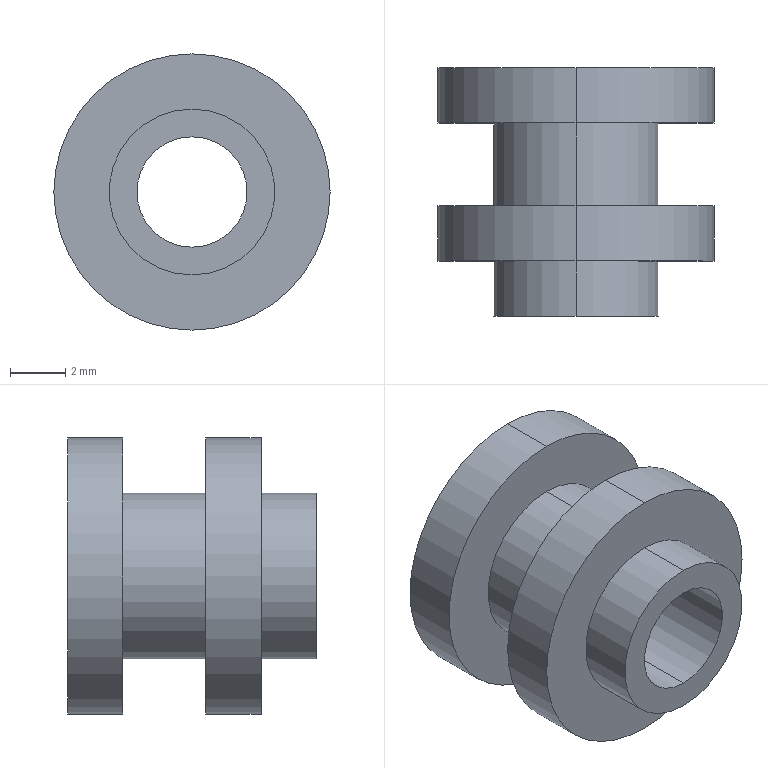Part | SolidWorks | features Extrusion 1, ICE 1, RevCut 1 | 1 solid | 15 faces | box 10 x 9 x 10 mm | volume 342.434 mm3 | cylinder 10 | plane 5 | commonest cylinder face diameters 6 x4 10 x4 4 x2
STEP:
#1=CARTESIAN_POINT('',(0.,0.,-2.));
#2=VERTEX_POINT('',#1);
#3=CARTESIAN_POINT('',(0.,0.,2.));
#4=VERTEX_POINT('',#3);
#5=CARTESIAN_POINT('',(0.,0.,0.));
#6=DIRECTION('',(0.,1.,0.));
#7=DIRECTION('',(0.,0.,1.));
#8=AXIS2_PLACEMENT_3D('',#5,#6,#7);
#9=CIRCLE('',#8,2.);
#10=EDGE_CURVE('',#2,#4,#9,.T.);
#11=ORIENTED_EDGE('',*,*,#10,.F.);
#12=CARTESIAN_POINT('',(0.,9.,-2.));
#13=VERTEX_POINT('',#12);
#14=CARTESIAN_POINT('',(0.,0.,-2.));
#15=DIRECTION('',(0.,1.,0.));
#16=VECTOR('',#15,1000.);
#17=LINE('',#14,#16);
#18=EDGE_CURVE('',#2,#13,#17,.T.);
#19=ORIENTED_EDGE('',*,*,#18,.T.);
#20=CARTESIAN_POINT('',(0.,9.,2.));
#21=VERTEX_POINT('',#20);
#22=CARTESIAN_POINT('',(0.,9.,0.));
#23=DIRECTION('',(0.,1.,0.));
#24=DIRECTION('',(0.,0.,1.));
#25=AXIS2_PLACEMENT_3D('',#22,#23,#24);
#26=CIRCLE('',#25,2.);
#27=EDGE_CURVE('',#13,#21,#26,.T.);
#28=ORIENTED_EDGE('',*,*,#27,.T.);
#29=CARTESIAN_POINT('',(0.,0.,2.));
#30=DIRECTION('',(0.,1.,0.));
#31=VECTOR('',#30,1000.);
#32=LINE('',#29,#31);
#33=EDGE_CURVE('',#4,#21,#32,.T.);
#34=ORIENTED_EDGE('',*,*,#33,.F.);
#35=EDGE_LOOP('',(#11,#19,#28,#34));
#36=FACE_OUTER_BOUND('',#35,.T.);
#37=CARTESIAN_POINT('',(0.,0.,0.));
#38=DIRECTION('',(0.,1.,0.));
#39=DIRECTION('',(0.,0.,1.));
#40=AXIS2_PLACEMENT_3D('',#37,#38,#39);
#41=CYLINDRICAL_SURFACE('',#40,2.);
#42=ADVANCED_FACE('',(#36),#41,.F.);
#43=CARTESIAN_POINT('',(0.,2.,-3.));
#44=VERTEX_POINT('',#43);
#45=CARTESIAN_POINT('',(0.,2.,3.));
#46=VERTEX_POINT('',#45);
#47=CARTESIAN_POINT('',(0.,2.,0.));
#48=DIRECTION('',(0.,-1.,0.));
#49=DIRECTION('',(0.,0.,-1.));
#50=AXIS2_PLACEMENT_3D('',#47,#48,#49);
#51=CIRCLE('',#50,3.);
#52=EDGE_CURVE('',#44,#46,#51,.T.);
#53=ORIENTED_EDGE('',*,*,#52,.T.);
#54=CARTESIAN_POINT('',(0.,0.,3.));
#55=VERTEX_POINT('',#54);
#56=CARTESIAN_POINT('',(0.,0.,3.));
#57=DIRECTION('',(0.,-1.,0.));
#58=VECTOR('',#57,1000.);
#59=LINE('',#56,#58);
#60=EDGE_CURVE('',#46,#55,#59,.T.);
#61=ORIENTED_EDGE('',*,*,#60,.T.);
#62=CARTESIAN_POINT('',(0.,0.,-3.));
#63=VERTEX_POINT('',#62);
#64=CARTESIAN_POINT('',(0.,0.,0.));
#65=DIRECTION('',(0.,-1.,0.));
#66=DIRECTION('',(0.,0.,-1.));
#67=AXIS2_PLACEMENT_3D('',#64,#65,#66);
#68=CIRCLE('',#67,3.);
#69=EDGE_CURVE('',#63,#55,#68,.T.);
#70=ORIENTED_EDGE('',*,*,#69,.F.);
#71=CARTESIAN_POINT('',(0.,0.,-3.));
#72=DIRECTION('',(0.,-1.,0.));
#73=VECTOR('',#72,1000.);
#74=LINE('',#71,#73);
#75=EDGE_CURVE('',#44,#63,#74,.T.);
#76=ORIENTED_EDGE('',*,*,#75,.F.);
#77=EDGE_LOOP('',(#53,#61,#70,#76));
#78=FACE_OUTER_BOUND('',#77,.T.);
#79=CARTESIAN_POINT('',(0.,0.,0.));
#80=DIRECTION('',(0.,-1.,0.));
#81=DIRECTION('',(0.,0.,-1.));
#82=AXIS2_PLACEMENT_3D('',#79,#80,#81);
#83=CYLINDRICAL_SURFACE('',#82,3.);
#84=ADVANCED_FACE('',(#78),#83,.T.);
#85=CARTESIAN_POINT('',(0.,4.,-5.));
#86=VERTEX_POINT('',#85);
#87=CARTESIAN_POINT('',(0.,4.,5.));
#88=VERTEX_POINT('',#87);
#89=CARTESIAN_POINT('',(0.,4.,0.));
#90=DIRECTION('',(0.,-1.,0.));
#91=DIRECTION('',(0.,0.,-1.));
#92=AXIS2_PLACEMENT_3D('',#89,#90,#91);
#93=CIRCLE('',#92,5.);
#94=EDGE_CURVE('',#86,#88,#93,.T.);
#95=ORIENTED_EDGE('',*,*,#94,.T.);
#96=CARTESIAN_POINT('',(0.,2.,5.));
#97=VERTEX_POINT('',#96);
#98=CARTESIAN_POINT('',(0.,9.,5.));
#99=DIRECTION('',(0.,-1.,0.));
#100=VECTOR('',#99,1000.);
#101=LINE('',#98,#100);
#102=EDGE_CURVE('',#88,#97,#101,.T.);
#103=ORIENTED_EDGE('',*,*,#102,.T.);
#104=CARTESIAN_POINT('',(0.,2.,-5.));
#105=VERTEX_POINT('',#104);
#106=CARTESIAN_POINT('',(0.,2.,0.));
#107=DIRECTION('',(0.,-1.,0.));
#108=DIRECTION('',(0.,0.,-1.));
#109=AXIS2_PLACEMENT_3D('',#106,#107,#108);
#110=CIRCLE('',#109,5.);
#111=EDGE_CURVE('',#105,#97,#110,.T.);
#112=ORIENTED_EDGE('',*,*,#111,.F.);
#113=CARTESIAN_POINT('',(0.,9.,-5.));
#114=DIRECTION('',(0.,-1.,0.));
#115=VECTOR('',#114,1000.);
#116=LINE('',#113,#115);
#117=EDGE_CURVE('',#86,#105,#116,.T.);
#118=ORIENTED_EDGE('',*,*,#117,.F.);
#119=EDGE_LOOP('',(#95,#103,#112,#118));
#120=FACE_OUTER_BOUND('',#119,.T.);
#121=CARTESIAN_POINT('',(0.,9.,0.));
#122=DIRECTION('',(0.,-1.,0.));
#123=DIRECTION('',(0.,0.,-1.));
#124=AXIS2_PLACEMENT_3D('',#121,#122,#123);
#125=CYLINDRICAL_SURFACE('',#124,5.);
#126=ADVANCED_FACE('',(#120),#125,.T.);
#127=CARTESIAN_POINT('',(0.,7.,-3.));
#128=VERTEX_POINT('',#127);
#129=CARTESIAN_POINT('',(0.,7.,3.));
#130=VERTEX_POINT('',#129);
#131=CARTESIAN_POINT('',(0.,7.,0.));
#132=DIRECTION('',(0.,-1.,0.));
#133=DIRECTION('',(0.,0.,-1.));
#134=AXIS2_PLACEMENT_3D('',#131,#132,#133);
#135=CIRCLE('',#134,3.);
#136=EDGE_CURVE('',#128,#130,#135,.T.);
#137=ORIENTED_EDGE('',*,*,#136,.T.);
#138=CARTESIAN_POINT('',(0.,4.,3.));
#139=VERTEX_POINT('',#138);
#140=CARTESIAN_POINT('',(0.,0.,3.));
#141=DIRECTION('',(0.,-1.,0.));
#142=VECTOR('',#141,1000.);
#143=LINE('',#140,#142);
#144=EDGE_CURVE('',#130,#139,#143,.T.);
#145=ORIENTED_EDGE('',*,*,#144,.T.);
#146=CARTESIAN_POINT('',(0.,4.,-3.));
#147=VERTEX_POINT('',#146);
#148=CARTESIAN_POINT('',(0.,4.,0.));
#149=DIRECTION('',(0.,-1.,0.));
#150=DIRECTION('',(0.,0.,-1.));
#151=AXIS2_PLACEMENT_3D('',#148,#149,#150);
#152=CIRCLE('',#151,3.);
#153=EDGE_CURVE('',#147,#139,#152,.T.);
#154=ORIENTED_EDGE('',*,*,#153,.F.);
#155=CARTESIAN_POINT('',(0.,0.,-3.));
#156=DIRECTION('',(0.,-1.,0.));
#157=VECTOR('',#156,1000.);
#158=LINE('',#155,#157);
#159=EDGE_CURVE('',#128,#147,#158,.T.);
#160=ORIENTED_EDGE('',*,*,#159,.F.);
#161=EDGE_LOOP('',(#137,#145,#154,#160));
#162=FACE_OUTER_BOUND('',#161,.T.);
#163=CARTESIAN_POINT('',(0.,0.,0.));
#164=DIRECTION('',(0.,-1.,0.));
#165=DIRECTION('',(0.,0.,-1.));
#166=AXIS2_PLACEMENT_3D('',#163,#164,#165);
#167=CYLINDRICAL_SURFACE('',#166,3.);
#168=ADVANCED_FACE('',(#162),#167,.T.);
#169=CARTESIAN_POINT('',(0.,9.,5.));
#170=VERTEX_POINT('',#169);
#171=CARTESIAN_POINT('',(0.,9.,-5.));
#172=VERTEX_POINT('',#171);
#173=CARTESIAN_POINT('',(0.,9.,0.));
#174=DIRECTION('',(0.,1.,0.));
#175=DIRECTION('',(0.,0.,1.));
#176=AXIS2_PLACEMENT_3D('',#173,#174,#175);
#177=CIRCLE('',#176,5.);
#178=EDGE_CURVE('',#170,#172,#177,.T.);
#179=ORIENTED_EDGE('',*,*,#178,.F.);
#180=CARTESIAN_POINT('',(0.,7.,5.));
#181=VERTEX_POINT('',#180);
#182=CARTESIAN_POINT('',(0.,9.,5.));
#183=DIRECTION('',(0.,-1.,0.));
#184=VECTOR('',#183,1000.);
#185=LINE('',#182,#184);
#186=EDGE_CURVE('',#170,#181,#185,.T.);
#187=ORIENTED_EDGE('',*,*,#186,.T.);
#188=CARTESIAN_POINT('',(0.,7.,-5.));
#189=VERTEX_POINT('',#188);
#190=CARTESIAN_POINT('',(0.,7.,0.));
#191=DIRECTION('',(0.,-1.,0.));
#192=DIRECTION('',(0.,0.,-1.));
#193=AXIS2_PLACEMENT_3D('',#190,#191,#192);
#194=CIRCLE('',#193,5.);
#195=EDGE_CURVE('',#189,#181,#194,.T.);
#196=ORIENTED_EDGE('',*,*,#195,.F.);
#197=CARTESIAN_POINT('',(0.,9.,-5.));
#198=DIRECTION('',(0.,-1.,0.));
#199=VECTOR('',#198,1000.);
#200=LINE('',#197,#199);
#201=EDGE_CURVE('',#172,#189,#200,.T.);
#202=ORIENTED_EDGE('',*,*,#201,.F.);
#203=EDGE_LOOP('',(#179,#187,#196,#202));
#204=FACE_OUTER_BOUND('',#203,.T.);
#205=CARTESIAN_POINT('',(0.,9.,0.));
#206=DIRECTION('',(0.,-1.,0.));
#207=DIRECTION('',(0.,0.,-1.));
#208=AXIS2_PLACEMENT_3D('',#205,#206,#207);
#209=CYLINDRICAL_SURFACE('',#208,5.);
#210=ADVANCED_FACE('',(#204),#209,.T.);
#211=ORIENTED_EDGE('',*,*,#186,.F.);
#212=CARTESIAN_POINT('',(0.,9.,0.));
#213=DIRECTION('',(0.,1.,0.));
#214=DIRECTION('',(0.,0.,1.));
#215=AXIS2_PLACEMENT_3D('',#212,#213,#214);
#216=CIRCLE('',#215,5.);
#217=EDGE_CURVE('',#172,#170,#216,.T.);
#218=ORIENTED_EDGE('',*,*,#217,.F.);
#219=ORIENTED_EDGE('',*,*,#201,.T.);
#220=CARTESIAN_POINT('',(0.,7.,0.));
#221=DIRECTION('',(0.,-1.,0.));
#222=DIRECTION('',(0.,0.,-1.));
#223=AXIS2_PLACEMENT_3D('',#220,#221,#222);
#224=CIRCLE('',#223,5.);
#225=EDGE_CURVE('',#181,#189,#224,.T.);
#226=ORIENTED_EDGE('',*,*,#225,.F.);
#227=EDGE_LOOP('',(#211,#218,#219,#226));
#228=FACE_OUTER_BOUND('',#227,.T.);
#229=CARTESIAN_POINT('',(0.,9.,0.));
#230=DIRECTION('',(0.,-1.,0.));
#231=DIRECTION('',(0.,0.,-1.));
#232=AXIS2_PLACEMENT_3D('',#229,#230,#231);
#233=CYLINDRICAL_SURFACE('',#232,5.);
#234=ADVANCED_FACE('',(#228),#233,.T.);
#235=CARTESIAN_POINT('',(0.,9.,0.));
#236=DIRECTION('',(0.,1.,0.));
#237=DIRECTION('',(0.,0.,1.));
#238=AXIS2_PLACEMENT_3D('',#235,#236,#237);
#239=CIRCLE('',#238,2.);
#240=EDGE_CURVE('',#21,#13,#239,.T.);
#241=ORIENTED_EDGE('',*,*,#240,.F.);
#242=ORIENTED_EDGE('',*,*,#27,.F.);
#243=EDGE_LOOP('',(#241,#242));
#244=FACE_BOUND('',#243,.T.);
#245=ORIENTED_EDGE('',*,*,#217,.T.);
#246=ORIENTED_EDGE('',*,*,#178,.T.);
#247=EDGE_LOOP('',(#245,#246));
#248=FACE_OUTER_BOUND('',#247,.T.);
#249=CARTESIAN_POINT('',(0.,9.,0.));
#250=DIRECTION('',(0.,1.,0.));
#251=DIRECTION('',(0.,0.,1.));
#252=AXIS2_PLACEMENT_3D('',#249,#250,#251);
#253=PLANE('',#252);
#254=ADVANCED_FACE('',(#244,#248),#253,.T.);
#255=ORIENTED_EDGE('',*,*,#94,.F.);
#256=CARTESIAN_POINT('',(0.,4.,0.));
#257=DIRECTION('',(0.,-1.,0.));
#258=DIRECTION('',(0.,0.,-1.));
#259=AXIS2_PLACEMENT_3D('',#256,#257,#258);
#260=CIRCLE('',#259,5.);
#261=EDGE_CURVE('',#88,#86,#260,.T.);
#262=ORIENTED_EDGE('',*,*,#261,.F.);
#263=EDGE_LOOP('',(#255,#262));
#264=FACE_OUTER_BOUND('',#263,.T.);
#265=ORIENTED_EDGE('',*,*,#153,.T.);
#266=CARTESIAN_POINT('',(0.,4.,0.));
#267=DIRECTION('',(0.,-1.,0.));
#268=DIRECTION('',(0.,0.,-1.));
#269=AXIS2_PLACEMENT_3D('',#266,#267,#268);
#270=CIRCLE('',#269,3.);
#271=EDGE_CURVE('',#139,#147,#270,.T.);
#272=ORIENTED_EDGE('',*,*,#271,.T.);
#273=EDGE_LOOP('',(#265,#272));
#274=FACE_BOUND('',#273,.T.);
#275=CARTESIAN_POINT('',(5.,4.,0.));
#276=DIRECTION('',(0.,-1.,0.));
#277=DIRECTION('',(0.,0.,-1.));
#278=AXIS2_PLACEMENT_3D('',#275,#276,#277);
#279=PLANE('',#278);
#280=ADVANCED_FACE('',(#264,#274),#279,.F.);
#281=ORIENTED_EDGE('',*,*,#144,.F.);
#282=CARTESIAN_POINT('',(0.,7.,0.));
#283=DIRECTION('',(0.,-1.,0.));
#284=DIRECTION('',(0.,0.,-1.));
#285=AXIS2_PLACEMENT_3D('',#282,#283,#284);
#286=CIRCLE('',#285,3.);
#287=EDGE_CURVE('',#130,#128,#286,.T.);
#288=ORIENTED_EDGE('',*,*,#287,.T.);
#289=ORIENTED_EDGE('',*,*,#159,.T.);
#290=ORIENTED_EDGE('',*,*,#271,.F.);
#291=EDGE_LOOP('',(#281,#288,#289,#290));
#292=FACE_OUTER_BOUND('',#291,.T.);
#293=CARTESIAN_POINT('',(0.,0.,0.));
#294=DIRECTION('',(0.,-1.,0.));
#295=DIRECTION('',(0.,0.,-1.));
#296=AXIS2_PLACEMENT_3D('',#293,#294,#295);
#297=CYLINDRICAL_SURFACE('',#296,3.);
#298=ADVANCED_FACE('',(#292),#297,.T.);
#299=ORIENTED_EDGE('',*,*,#136,.F.);
#300=ORIENTED_EDGE('',*,*,#287,.F.);
#301=EDGE_LOOP('',(#299,#300));
#302=FACE_BOUND('',#301,.T.);
#303=ORIENTED_EDGE('',*,*,#195,.T.);
#304=ORIENTED_EDGE('',*,*,#225,.T.);
#305=EDGE_LOOP('',(#303,#304));
#306=FACE_OUTER_BOUND('',#305,.T.);
#307=CARTESIAN_POINT('',(5.,7.,0.));
#308=DIRECTION('',(0.,1.,0.));
#309=DIRECTION('',(0.,0.,1.));
#310=AXIS2_PLACEMENT_3D('',#307,#308,#309);
#311=PLANE('',#310);
#312=ADVANCED_FACE('',(#302,#306),#311,.F.);
#313=ORIENTED_EDGE('',*,*,#102,.F.);
#314=ORIENTED_EDGE('',*,*,#261,.T.);
#315=ORIENTED_EDGE('',*,*,#117,.T.);
#316=CARTESIAN_POINT('',(0.,2.,0.));
#317=DIRECTION('',(0.,-1.,0.));
#318=DIRECTION('',(0.,0.,-1.));
#319=AXIS2_PLACEMENT_3D('',#316,#317,#318);
#320=CIRCLE('',#319,5.);
#321=EDGE_CURVE('',#97,#105,#320,.T.);
#322=ORIENTED_EDGE('',*,*,#321,.F.);
#323=EDGE_LOOP('',(#313,#314,#315,#322));
#324=FACE_OUTER_BOUND('',#323,.T.);
#325=CARTESIAN_POINT('',(0.,9.,0.));
#326=DIRECTION('',(0.,-1.,0.));
#327=DIRECTION('',(0.,0.,-1.));
#328=AXIS2_PLACEMENT_3D('',#325,#326,#327);
#329=CYLINDRICAL_SURFACE('',#328,5.);
#330=ADVANCED_FACE('',(#324),#329,.T.);
#331=ORIENTED_EDGE('',*,*,#52,.F.);
#332=CARTESIAN_POINT('',(0.,2.,0.));
#333=DIRECTION('',(0.,-1.,0.));
#334=DIRECTION('',(0.,0.,-1.));
#335=AXIS2_PLACEMENT_3D('',#332,#333,#334);
#336=CIRCLE('',#335,3.);
#337=EDGE_CURVE('',#46,#44,#336,.T.);
#338=ORIENTED_EDGE('',*,*,#337,.F.);
#339=EDGE_LOOP('',(#331,#338));
#340=FACE_BOUND('',#339,.T.);
#341=ORIENTED_EDGE('',*,*,#111,.T.);
#342=ORIENTED_EDGE('',*,*,#321,.T.);
#343=EDGE_LOOP('',(#341,#342));
#344=FACE_OUTER_BOUND('',#343,.T.);
#345=CARTESIAN_POINT('',(5.,2.,0.));
#346=DIRECTION('',(0.,1.,0.));
#347=DIRECTION('',(0.,0.,1.));
#348=AXIS2_PLACEMENT_3D('',#345,#346,#347);
#349=PLANE('',#348);
#350=ADVANCED_FACE('',(#340,#344),#349,.F.);
#351=ORIENTED_EDGE('',*,*,#60,.F.);
#352=ORIENTED_EDGE('',*,*,#337,.T.);
#353=ORIENTED_EDGE('',*,*,#75,.T.);
#354=CARTESIAN_POINT('',(0.,0.,0.));
#355=DIRECTION('',(0.,-1.,0.));
#356=DIRECTION('',(0.,0.,-1.));
#357=AXIS2_PLACEMENT_3D('',#354,#355,#356);
#358=CIRCLE('',#357,3.);
#359=EDGE_CURVE('',#55,#63,#358,.T.);
#360=ORIENTED_EDGE('',*,*,#359,.F.);
#361=EDGE_LOOP('',(#351,#352,#353,#360));
#362=FACE_OUTER_BOUND('',#361,.T.);
#363=CARTESIAN_POINT('',(0.,0.,0.));
#364=DIRECTION('',(0.,-1.,0.));
#365=DIRECTION('',(0.,0.,-1.));
#366=AXIS2_PLACEMENT_3D('',#363,#364,#365);
#367=CYLINDRICAL_SURFACE('',#366,3.);
#368=ADVANCED_FACE('',(#362),#367,.T.);
#369=CARTESIAN_POINT('',(0.,0.,0.));
#370=DIRECTION('',(0.,1.,0.));
#371=DIRECTION('',(0.,0.,1.));
#372=AXIS2_PLACEMENT_3D('',#369,#370,#371);
#373=CIRCLE('',#372,2.);
#374=EDGE_CURVE('',#4,#2,#373,.T.);
#375=ORIENTED_EDGE('',*,*,#374,.T.);
#376=ORIENTED_EDGE('',*,*,#10,.T.);
#377=EDGE_LOOP('',(#375,#376));
#378=FACE_BOUND('',#377,.T.);
#379=ORIENTED_EDGE('',*,*,#69,.T.);
#380=ORIENTED_EDGE('',*,*,#359,.T.);
#381=EDGE_LOOP('',(#379,#380));
#382=FACE_OUTER_BOUND('',#381,.T.);
#383=CARTESIAN_POINT('',(0.,0.,0.));
#384=DIRECTION('',(0.,1.,0.));
#385=DIRECTION('',(0.,0.,1.));
#386=AXIS2_PLACEMENT_3D('',#383,#384,#385);
#387=PLANE('',#386);
#388=ADVANCED_FACE('',(#378,#382),#387,.F.);
#389=ORIENTED_EDGE('',*,*,#18,.F.);
#390=ORIENTED_EDGE('',*,*,#374,.F.);
#391=ORIENTED_EDGE('',*,*,#33,.T.);
#392=ORIENTED_EDGE('',*,*,#240,.T.);
#393=EDGE_LOOP('',(#389,#390,#391,#392));
#394=FACE_OUTER_BOUND('',#393,.T.);
#395=CARTESIAN_POINT('',(0.,0.,0.));
#396=DIRECTION('',(0.,1.,0.));
#397=DIRECTION('',(0.,0.,1.));
#398=AXIS2_PLACEMENT_3D('',#395,#396,#397);
#399=CYLINDRICAL_SURFACE('',#398,2.);
#400=ADVANCED_FACE('',(#394),#399,.F.);
#401=CLOSED_SHELL('',(#42,#84,#126,#168,#210,#234,#254,#280,#298,#312,#330,#350,#368,#388,#400));
#402=MANIFOLD_SOLID_BREP('',#401);
#403=CARTESIAN_POINT('',(0.,0.,0.));
#404=DIRECTION('',(0.,0.,1.));
#405=DIRECTION('',(1.,0.,0.));
#406=AXIS2_PLACEMENT_3D('',#403,#404,#405);
#407=(LENGTH_UNIT()NAMED_UNIT(*)SI_UNIT(.MILLI.,.METRE.));
#408=UNCERTAINTY_MEASURE_WITH_UNIT(LENGTH_MEASURE(0.00001),#407,'','');
#409=(NAMED_UNIT(*)PLANE_ANGLE_UNIT()SI_UNIT($,.RADIAN.));
#410=(NAMED_UNIT(*)SI_UNIT($,.STERADIAN.)SOLID_ANGLE_UNIT());
#411=(GEOMETRIC_REPRESENTATION_CONTEXT(3)GLOBAL_UNCERTAINTY_ASSIGNED_CONTEXT((#408))GLOBAL_UNIT_ASSIGNED_CONTEXT((#407,#409,#410))REPRESENTATION_CONTEXT('',''));
#412=ADVANCED_BREP_SHAPE_REPRESENTATION('',(#402,#406),#411);